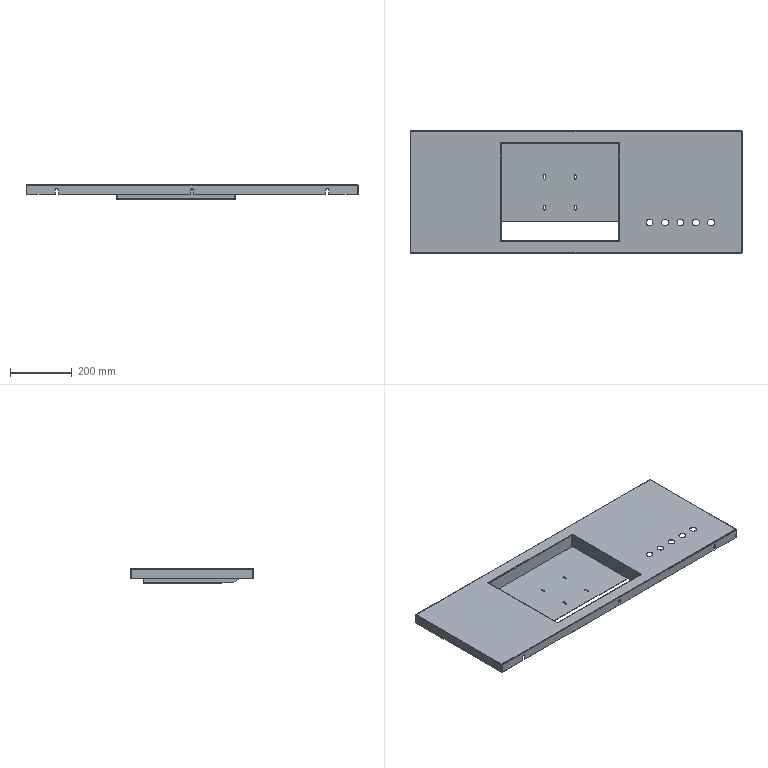Part | STEP file | 09-08 panel (Default) | 1 solid | 139 faces | box 1078 x 398 x 48 mm | volume 808105 mm3 | plane 74 | cylinder 49 | spline 16 | commonest cylinder face diameters 1.473 x10 4.473 x10 22 x10 8.5 x9 5 x8 60 x2